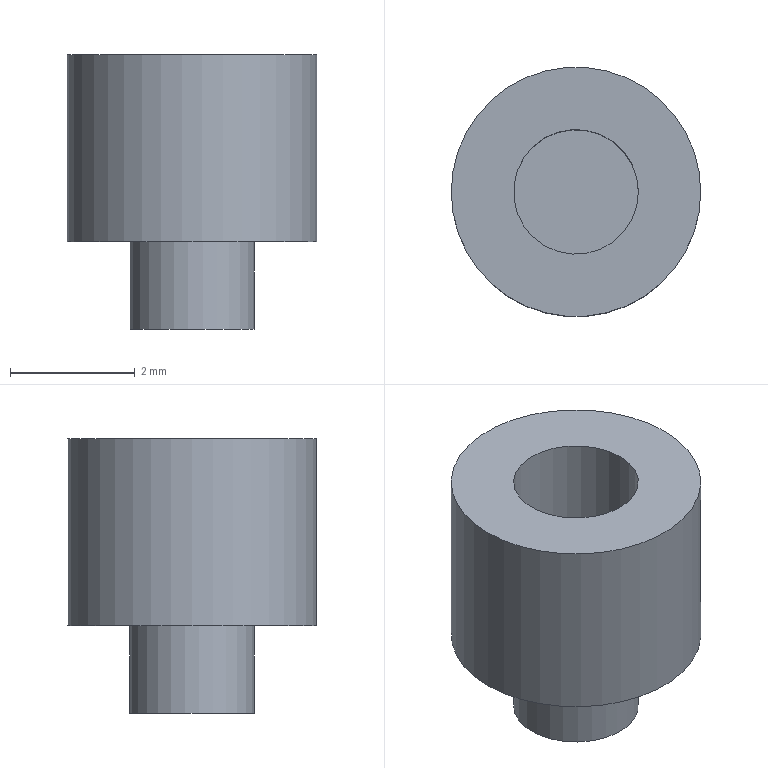Part | STEP file | Solder post | 2 solids | 7 faces | box 4 x 4 x 4.4 mm | volume 32.673 mm3 | plane 4 | cylinder 3 | commonest cylinder face diameters 2 x2 4 x1
STEP:
#1=CARTESIAN_POINT('',(0.,0.,0.));
#2=DIRECTION('',(0.,0.,1.));
#3=DIRECTION('',(1.,0.,0.));
#4=AXIS2_PLACEMENT_3D('',#1,#2,#3);
#5=CARTESIAN_POINT('',(2.,0.,3.));
#6=VERTEX_POINT('',#5);
#7=CARTESIAN_POINT('',(0.,0.,3.));
#8=DIRECTION('',(0.,0.,1.));
#9=DIRECTION('',(1.,0.,0.));
#10=AXIS2_PLACEMENT_3D('',#7,#8,#9);
#11=CIRCLE('',#10,2.);
#12=CARTESIAN_POINT('',(0.,0.,3.));
#13=DIRECTION('',(0.,0.,-1.));
#14=DIRECTION('',(-1.,0.,0.));
#15=AXIS2_PLACEMENT_3D('',#12,#13,#14);
#16=CYLINDRICAL_SURFACE('',#15,2.);
#17=CARTESIAN_POINT('',(9.425,0.));
#18=DIRECTION('',(-1.,0.));
#19=VECTOR('',#18,1.);
#20=LINE('',#17,#19);
#21=(GEOMETRIC_REPRESENTATION_CONTEXT(2)PARAMETRIC_REPRESENTATION_CONTEXT()REPRESENTATION_CONTEXT('',''));
#22=DEFINITIONAL_REPRESENTATION('',(#20),#21);
#23=PCURVE('',#16,#22);
#24=CARTESIAN_POINT('',(0.,0.,3.));
#25=DIRECTION('',(0.,0.,1.));
#26=DIRECTION('',(1.,0.,0.));
#27=AXIS2_PLACEMENT_3D('',#24,#25,#26);
#28=PLANE('',#27);
#29=CARTESIAN_POINT('',(0.,0.));
#30=DIRECTION('',(1.,0.));
#31=AXIS2_PLACEMENT_2D('',#29,#30);
#32=CIRCLE('',#31,2.);
#33=(GEOMETRIC_REPRESENTATION_CONTEXT(2)PARAMETRIC_REPRESENTATION_CONTEXT()REPRESENTATION_CONTEXT('',''));
#34=DEFINITIONAL_REPRESENTATION('',(#32),#33);
#35=PCURVE('',#28,#34);
#36=SURFACE_CURVE('',#11,(#23,#35),.PCURVE_S1.);
#37=EDGE_CURVE('',#6,#6,#36,.T.);
#38=ORIENTED_EDGE('',*,*,#37,.F.);
#39=CARTESIAN_POINT('',(2.,0.,0.));
#40=VERTEX_POINT('',#39);
#41=CARTESIAN_POINT('',(2.,0.,3.));
#42=CARTESIAN_POINT('',(2.,0.,0.));
#43=B_SPLINE_CURVE_WITH_KNOTS('',1,(#41,#42),.UNSPECIFIED.,.F.,.F.,(2,2),(0.,3.),.PIECEWISE_BEZIER_KNOTS.);
#44=CARTESIAN_POINT('',(9.425,0.));
#45=DIRECTION('',(0.,1.));
#46=VECTOR('',#45,1.);
#47=LINE('',#44,#46);
#48=(GEOMETRIC_REPRESENTATION_CONTEXT(2)PARAMETRIC_REPRESENTATION_CONTEXT()REPRESENTATION_CONTEXT('',''));
#49=DEFINITIONAL_REPRESENTATION('',(#47),#48);
#50=PCURVE('',#16,#49);
#51=CARTESIAN_POINT('',(3.142,0.));
#52=DIRECTION('',(0.,1.));
#53=VECTOR('',#52,1.);
#54=LINE('',#51,#53);
#55=(GEOMETRIC_REPRESENTATION_CONTEXT(2)PARAMETRIC_REPRESENTATION_CONTEXT()REPRESENTATION_CONTEXT('',''));
#56=DEFINITIONAL_REPRESENTATION('',(#54),#55);
#57=PCURVE('',#16,#56);
#58=SEAM_CURVE('',#43,(#50,#57),.PCURVE_S1.);
#59=EDGE_CURVE('',#6,#40,#58,.T.);
#60=ORIENTED_EDGE('',*,*,#59,.T.);
#61=CARTESIAN_POINT('',(0.,0.,0.));
#62=DIRECTION('',(0.,0.,1.));
#63=DIRECTION('',(1.,0.,0.));
#64=AXIS2_PLACEMENT_3D('',#61,#62,#63);
#65=CIRCLE('',#64,2.);
#66=CARTESIAN_POINT('',(9.425,3.));
#67=DIRECTION('',(-1.,0.));
#68=VECTOR('',#67,1.);
#69=LINE('',#66,#68);
#70=(GEOMETRIC_REPRESENTATION_CONTEXT(2)PARAMETRIC_REPRESENTATION_CONTEXT()REPRESENTATION_CONTEXT('',''));
#71=DEFINITIONAL_REPRESENTATION('',(#69),#70);
#72=PCURVE('',#16,#71);
#73=CARTESIAN_POINT('',(0.,0.,0.));
#74=DIRECTION('',(0.,0.,1.));
#75=DIRECTION('',(1.,0.,0.));
#76=AXIS2_PLACEMENT_3D('',#73,#74,#75);
#77=PLANE('',#76);
#78=CARTESIAN_POINT('',(0.,0.));
#79=DIRECTION('',(1.,0.));
#80=AXIS2_PLACEMENT_2D('',#78,#79);
#81=CIRCLE('',#80,2.);
#82=(GEOMETRIC_REPRESENTATION_CONTEXT(2)PARAMETRIC_REPRESENTATION_CONTEXT()REPRESENTATION_CONTEXT('',''));
#83=DEFINITIONAL_REPRESENTATION('',(#81),#82);
#84=PCURVE('',#77,#83);
#85=SURFACE_CURVE('',#65,(#72,#84),.PCURVE_S1.);
#86=EDGE_CURVE('',#40,#40,#85,.T.);
#87=ORIENTED_EDGE('',*,*,#86,.T.);
#88=ORIENTED_EDGE('',*,*,#59,.F.);
#89=EDGE_LOOP('',(#38,#60,#87,#88));
#90=FACE_BOUND('',#89,.T.);
#91=ADVANCED_FACE('',(#90),#16,.T.);
#92=CARTESIAN_POINT('',(1.,0.,3.));
#93=VERTEX_POINT('',#92);
#94=CARTESIAN_POINT('',(0.,0.,3.));
#95=DIRECTION('',(0.,0.,1.));
#96=DIRECTION('',(1.,0.,0.));
#97=AXIS2_PLACEMENT_3D('',#94,#95,#96);
#98=CIRCLE('',#97,1.);
#99=CARTESIAN_POINT('',(0.,0.,3.));
#100=DIRECTION('',(0.,0.,-1.));
#101=DIRECTION('',(-1.,0.,0.));
#102=AXIS2_PLACEMENT_3D('',#99,#100,#101);
#103=CYLINDRICAL_SURFACE('',#102,1.);
#104=CARTESIAN_POINT('',(9.425,0.));
#105=DIRECTION('',(-1.,0.));
#106=VECTOR('',#105,1.);
#107=LINE('',#104,#106);
#108=(GEOMETRIC_REPRESENTATION_CONTEXT(2)PARAMETRIC_REPRESENTATION_CONTEXT()REPRESENTATION_CONTEXT('',''));
#109=DEFINITIONAL_REPRESENTATION('',(#107),#108);
#110=PCURVE('',#103,#109);
#111=CARTESIAN_POINT('',(0.,0.));
#112=DIRECTION('',(1.,0.));
#113=AXIS2_PLACEMENT_2D('',#111,#112);
#114=CIRCLE('',#113,1.);
#115=(GEOMETRIC_REPRESENTATION_CONTEXT(2)PARAMETRIC_REPRESENTATION_CONTEXT()REPRESENTATION_CONTEXT('',''));
#116=DEFINITIONAL_REPRESENTATION('',(#114),#115);
#117=PCURVE('',#28,#116);
#118=SURFACE_CURVE('',#98,(#110,#117),.PCURVE_S1.);
#119=EDGE_CURVE('',#93,#93,#118,.T.);
#120=ORIENTED_EDGE('',*,*,#119,.F.);
#121=CARTESIAN_POINT('',(1.,0.,0.));
#122=VERTEX_POINT('',#121);
#123=CARTESIAN_POINT('',(1.,0.,3.));
#124=CARTESIAN_POINT('',(1.,0.,0.));
#125=B_SPLINE_CURVE_WITH_KNOTS('',1,(#123,#124),.UNSPECIFIED.,.F.,.F.,(2,2),(0.,3.),.PIECEWISE_BEZIER_KNOTS.);
#126=CARTESIAN_POINT('',(9.425,0.));
#127=DIRECTION('',(0.,1.));
#128=VECTOR('',#127,1.);
#129=LINE('',#126,#128);
#130=(GEOMETRIC_REPRESENTATION_CONTEXT(2)PARAMETRIC_REPRESENTATION_CONTEXT()REPRESENTATION_CONTEXT('',''));
#131=DEFINITIONAL_REPRESENTATION('',(#129),#130);
#132=PCURVE('',#103,#131);
#133=CARTESIAN_POINT('',(3.142,0.));
#134=DIRECTION('',(0.,1.));
#135=VECTOR('',#134,1.);
#136=LINE('',#133,#135);
#137=(GEOMETRIC_REPRESENTATION_CONTEXT(2)PARAMETRIC_REPRESENTATION_CONTEXT()REPRESENTATION_CONTEXT('',''));
#138=DEFINITIONAL_REPRESENTATION('',(#136),#137);
#139=PCURVE('',#103,#138);
#140=SEAM_CURVE('',#125,(#132,#139),.PCURVE_S1.);
#141=EDGE_CURVE('',#93,#122,#140,.T.);
#142=ORIENTED_EDGE('',*,*,#141,.T.);
#143=CARTESIAN_POINT('',(0.,0.,0.));
#144=DIRECTION('',(0.,0.,1.));
#145=DIRECTION('',(1.,0.,0.));
#146=AXIS2_PLACEMENT_3D('',#143,#144,#145);
#147=CIRCLE('',#146,1.);
#148=CARTESIAN_POINT('',(9.425,3.));
#149=DIRECTION('',(-1.,0.));
#150=VECTOR('',#149,1.);
#151=LINE('',#148,#150);
#152=(GEOMETRIC_REPRESENTATION_CONTEXT(2)PARAMETRIC_REPRESENTATION_CONTEXT()REPRESENTATION_CONTEXT('',''));
#153=DEFINITIONAL_REPRESENTATION('',(#151),#152);
#154=PCURVE('',#103,#153);
#155=CARTESIAN_POINT('',(0.,0.));
#156=DIRECTION('',(1.,0.));
#157=AXIS2_PLACEMENT_2D('',#155,#156);
#158=CIRCLE('',#157,1.);
#159=(GEOMETRIC_REPRESENTATION_CONTEXT(2)PARAMETRIC_REPRESENTATION_CONTEXT()REPRESENTATION_CONTEXT('',''));
#160=DEFINITIONAL_REPRESENTATION('',(#158),#159);
#161=PCURVE('',#77,#160);
#162=SURFACE_CURVE('',#147,(#154,#161),.PCURVE_S1.);
#163=EDGE_CURVE('',#122,#122,#162,.T.);
#164=ORIENTED_EDGE('',*,*,#163,.T.);
#165=ORIENTED_EDGE('',*,*,#141,.F.);
#166=EDGE_LOOP('',(#120,#142,#164,#165));
#167=FACE_BOUND('',#166,.F.);
#168=ADVANCED_FACE('',(#167),#103,.F.);
#169=ORIENTED_EDGE('',*,*,#37,.T.);
#170=EDGE_LOOP('',(#169));
#171=FACE_BOUND('',#170,.T.);
#172=ORIENTED_EDGE('',*,*,#119,.F.);
#173=EDGE_LOOP('',(#172));
#174=FACE_BOUND('',#173,.T.);
#175=ADVANCED_FACE('',(#171,#174),#28,.T.);
#176=ORIENTED_EDGE('',*,*,#86,.F.);
#177=EDGE_LOOP('',(#176));
#178=FACE_BOUND('',#177,.T.);
#179=ORIENTED_EDGE('',*,*,#163,.T.);
#180=EDGE_LOOP('',(#179));
#181=FACE_BOUND('',#180,.T.);
#182=ADVANCED_FACE('',(#178,#181),#77,.F.);
#183=CLOSED_SHELL('',(#91,#168,#175,#182));
#184=MANIFOLD_SOLID_BREP('',#183);
#185=CARTESIAN_POINT('',(1.,0.,-1.4));
#186=VERTEX_POINT('',#185);
#187=CARTESIAN_POINT('',(0.,0.,-1.4));
#188=DIRECTION('',(0.,0.,-1.));
#189=DIRECTION('',(1.,0.,0.));
#190=AXIS2_PLACEMENT_3D('',#187,#188,#189);
#191=CIRCLE('',#190,1.);
#192=CARTESIAN_POINT('',(0.,0.,-1.4));
#193=DIRECTION('',(0.,0.,1.));
#194=DIRECTION('',(1.,0.,0.));
#195=AXIS2_PLACEMENT_3D('',#192,#193,#194);
#196=CYLINDRICAL_SURFACE('',#195,1.);
#197=CARTESIAN_POINT('',(6.283,0.));
#198=DIRECTION('',(-1.,0.));
#199=VECTOR('',#198,1.);
#200=LINE('',#197,#199);
#201=(GEOMETRIC_REPRESENTATION_CONTEXT(2)PARAMETRIC_REPRESENTATION_CONTEXT()REPRESENTATION_CONTEXT('',''));
#202=DEFINITIONAL_REPRESENTATION('',(#200),#201);
#203=PCURVE('',#196,#202);
#204=CARTESIAN_POINT('',(0.,0.,-1.4));
#205=DIRECTION('',(0.,0.,-1.));
#206=DIRECTION('',(-1.,0.,0.));
#207=AXIS2_PLACEMENT_3D('',#204,#205,#206);
#208=PLANE('',#207);
#209=CARTESIAN_POINT('',(0.,0.));
#210=DIRECTION('',(-1.,0.));
#211=AXIS2_PLACEMENT_2D('',#209,#210);
#212=CIRCLE('',#211,1.);
#213=(GEOMETRIC_REPRESENTATION_CONTEXT(2)PARAMETRIC_REPRESENTATION_CONTEXT()REPRESENTATION_CONTEXT('',''));
#214=DEFINITIONAL_REPRESENTATION('',(#212),#213);
#215=PCURVE('',#208,#214);
#216=SURFACE_CURVE('',#191,(#203,#215),.PCURVE_S1.);
#217=EDGE_CURVE('',#186,#186,#216,.T.);
#218=ORIENTED_EDGE('',*,*,#217,.F.);
#219=CARTESIAN_POINT('',(1.,0.,0.));
#220=VERTEX_POINT('',#219);
#221=CARTESIAN_POINT('',(1.,0.,-1.4));
#222=CARTESIAN_POINT('',(1.,0.,0.));
#223=B_SPLINE_CURVE_WITH_KNOTS('',1,(#221,#222),.UNSPECIFIED.,.F.,.F.,(2,2),(0.,1.4),.PIECEWISE_BEZIER_KNOTS.);
#224=CARTESIAN_POINT('',(6.283,0.));
#225=DIRECTION('',(0.,1.));
#226=VECTOR('',#225,1.);
#227=LINE('',#224,#226);
#228=(GEOMETRIC_REPRESENTATION_CONTEXT(2)PARAMETRIC_REPRESENTATION_CONTEXT()REPRESENTATION_CONTEXT('',''));
#229=DEFINITIONAL_REPRESENTATION('',(#227),#228);
#230=PCURVE('',#196,#229);
#231=CARTESIAN_POINT('',(0.,0.));
#232=DIRECTION('',(0.,1.));
#233=VECTOR('',#232,1.);
#234=LINE('',#231,#233);
#235=(GEOMETRIC_REPRESENTATION_CONTEXT(2)PARAMETRIC_REPRESENTATION_CONTEXT()REPRESENTATION_CONTEXT('',''));
#236=DEFINITIONAL_REPRESENTATION('',(#234),#235);
#237=PCURVE('',#196,#236);
#238=SEAM_CURVE('',#223,(#230,#237),.PCURVE_S1.);
#239=EDGE_CURVE('',#186,#220,#238,.T.);
#240=ORIENTED_EDGE('',*,*,#239,.T.);
#241=CARTESIAN_POINT('',(0.,0.,0.));
#242=DIRECTION('',(0.,0.,-1.));
#243=DIRECTION('',(1.,0.,0.));
#244=AXIS2_PLACEMENT_3D('',#241,#242,#243);
#245=CIRCLE('',#244,1.);
#246=CARTESIAN_POINT('',(6.283,1.4));
#247=DIRECTION('',(-1.,0.));
#248=VECTOR('',#247,1.);
#249=LINE('',#246,#248);
#250=(GEOMETRIC_REPRESENTATION_CONTEXT(2)PARAMETRIC_REPRESENTATION_CONTEXT()REPRESENTATION_CONTEXT('',''));
#251=DEFINITIONAL_REPRESENTATION('',(#249),#250);
#252=PCURVE('',#196,#251);
#253=CARTESIAN_POINT('',(0.,0.,0.));
#254=DIRECTION('',(0.,0.,-1.));
#255=DIRECTION('',(-1.,0.,0.));
#256=AXIS2_PLACEMENT_3D('',#253,#254,#255);
#257=PLANE('',#256);
#258=CARTESIAN_POINT('',(0.,0.));
#259=DIRECTION('',(-1.,0.));
#260=AXIS2_PLACEMENT_2D('',#258,#259);
#261=CIRCLE('',#260,1.);
#262=(GEOMETRIC_REPRESENTATION_CONTEXT(2)PARAMETRIC_REPRESENTATION_CONTEXT()REPRESENTATION_CONTEXT('',''));
#263=DEFINITIONAL_REPRESENTATION('',(#261),#262);
#264=PCURVE('',#257,#263);
#265=SURFACE_CURVE('',#245,(#252,#264),.PCURVE_S1.);
#266=EDGE_CURVE('',#220,#220,#265,.T.);
#267=ORIENTED_EDGE('',*,*,#266,.T.);
#268=ORIENTED_EDGE('',*,*,#239,.F.);
#269=EDGE_LOOP('',(#218,#240,#267,#268));
#270=FACE_BOUND('',#269,.T.);
#271=ADVANCED_FACE('',(#270),#196,.T.);
#272=ORIENTED_EDGE('',*,*,#217,.T.);
#273=EDGE_LOOP('',(#272));
#274=FACE_BOUND('',#273,.T.);
#275=ADVANCED_FACE('',(#274),#208,.T.);
#276=ORIENTED_EDGE('',*,*,#266,.F.);
#277=EDGE_LOOP('',(#276));
#278=FACE_BOUND('',#277,.T.);
#279=ADVANCED_FACE('',(#278),#257,.F.);
#280=CLOSED_SHELL('',(#271,#275,#279));
#281=MANIFOLD_SOLID_BREP('',#280);
#282=(LENGTH_UNIT()NAMED_UNIT(*)SI_UNIT(.MILLI.,.METRE.));
#283=UNCERTAINTY_MEASURE_WITH_UNIT(LENGTH_MEASURE(0.00001),#282,'','');
#284=(NAMED_UNIT(*)PLANE_ANGLE_UNIT()SI_UNIT($,.RADIAN.));
#285=(NAMED_UNIT(*)SI_UNIT($,.STERADIAN.)SOLID_ANGLE_UNIT());
#286=(GEOMETRIC_REPRESENTATION_CONTEXT(3)GLOBAL_UNCERTAINTY_ASSIGNED_CONTEXT((#283))GLOBAL_UNIT_ASSIGNED_CONTEXT((#282,#284,#285))REPRESENTATION_CONTEXT('',''));
#287=SHAPE_REPRESENTATION('',(#4,#184,#281),#286);